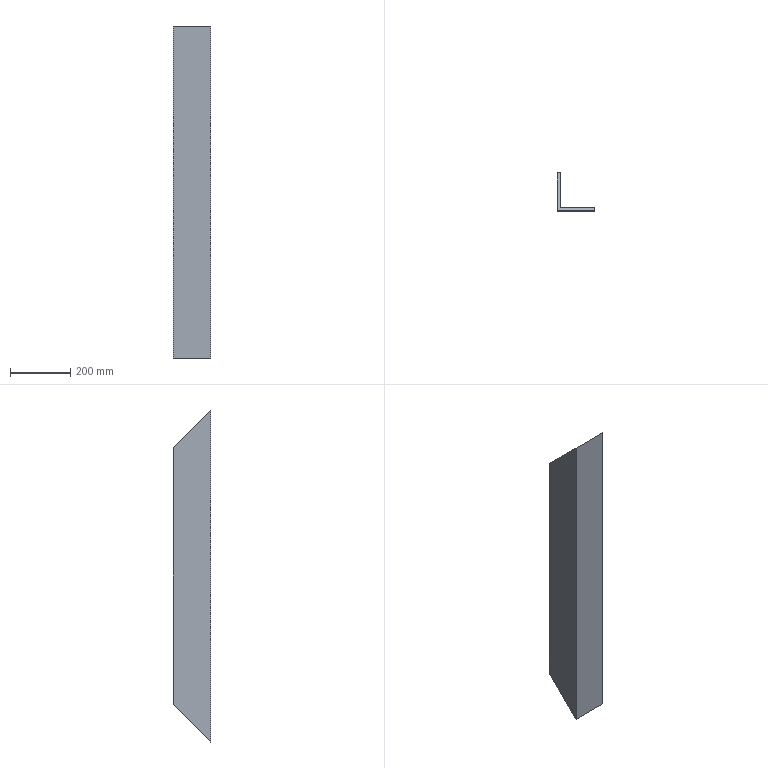Part | SolidWorks | features Extrusion 1, ICE 1 | 1 solid | 8 faces | box 125 x 125 x 1100 mm | volume 2472250 mm3 | plane 8
STEP:
#1=CARTESIAN_POINT('',(0.,125.,425.));
#2=VERTEX_POINT('',#1);
#3=CARTESIAN_POINT('',(10.,125.,425.));
#4=VERTEX_POINT('',#3);
#5=CARTESIAN_POINT('',(0.,125.,425.));
#6=DIRECTION('',(1.,0.,0.));
#7=VECTOR('',#6,1000.);
#8=LINE('',#5,#7);
#9=EDGE_CURVE('',#2,#4,#8,.T.);
#10=ORIENTED_EDGE('',*,*,#9,.T.);
#11=CARTESIAN_POINT('',(10.,125.,-425.));
#12=VERTEX_POINT('',#11);
#13=CARTESIAN_POINT('',(10.,125.,550.));
#14=DIRECTION('',(0.,0.,-1.));
#15=VECTOR('',#14,1000.);
#16=LINE('',#13,#15);
#17=EDGE_CURVE('',#4,#12,#16,.T.);
#18=ORIENTED_EDGE('',*,*,#17,.T.);
#19=CARTESIAN_POINT('',(0.,125.,-425.));
#20=VERTEX_POINT('',#19);
#21=CARTESIAN_POINT('',(0.,125.,-425.));
#22=DIRECTION('',(1.,0.,0.));
#23=VECTOR('',#22,1000.);
#24=LINE('',#21,#23);
#25=EDGE_CURVE('',#20,#12,#24,.T.);
#26=ORIENTED_EDGE('',*,*,#25,.F.);
#27=CARTESIAN_POINT('',(0.,125.,550.));
#28=DIRECTION('',(0.,0.,-1.));
#29=VECTOR('',#28,1000.);
#30=LINE('',#27,#29);
#31=EDGE_CURVE('',#2,#20,#30,.T.);
#32=ORIENTED_EDGE('',*,*,#31,.F.);
#33=EDGE_LOOP('',(#10,#18,#26,#32));
#34=FACE_OUTER_BOUND('',#33,.T.);
#35=CARTESIAN_POINT('',(0.,125.,550.));
#36=DIRECTION('',(0.,1.,0.));
#37=DIRECTION('',(0.,0.,1.));
#38=AXIS2_PLACEMENT_3D('',#35,#36,#37);
#39=PLANE('',#38);
#40=ADVANCED_FACE('',(#34),#39,.T.);
#41=CARTESIAN_POINT('',(0.,0.,550.));
#42=VERTEX_POINT('',#41);
#43=CARTESIAN_POINT('',(0.,0.,-550.));
#44=VERTEX_POINT('',#43);
#45=CARTESIAN_POINT('',(0.,0.,550.));
#46=DIRECTION('',(0.,0.,-1.));
#47=VECTOR('',#46,1000.);
#48=LINE('',#45,#47);
#49=EDGE_CURVE('',#42,#44,#48,.T.);
#50=ORIENTED_EDGE('',*,*,#49,.F.);
#51=CARTESIAN_POINT('',(0.,125.,425.));
#52=DIRECTION('',(0.,0.7071,-0.7071));
#53=VECTOR('',#52,1000.);
#54=LINE('',#51,#53);
#55=EDGE_CURVE('',#42,#2,#54,.T.);
#56=ORIENTED_EDGE('',*,*,#55,.T.);
#57=ORIENTED_EDGE('',*,*,#31,.T.);
#58=CARTESIAN_POINT('',(0.,125.,-425.));
#59=DIRECTION('',(0.,-0.7071,-0.7071));
#60=VECTOR('',#59,1000.);
#61=LINE('',#58,#60);
#62=EDGE_CURVE('',#20,#44,#61,.T.);
#63=ORIENTED_EDGE('',*,*,#62,.T.);
#64=EDGE_LOOP('',(#50,#56,#57,#63));
#65=FACE_OUTER_BOUND('',#64,.T.);
#66=CARTESIAN_POINT('',(0.,0.,550.));
#67=DIRECTION('',(1.,0.,0.));
#68=DIRECTION('',(0.,1.,0.));
#69=AXIS2_PLACEMENT_3D('',#66,#67,#68);
#70=PLANE('',#69);
#71=ADVANCED_FACE('',(#65),#70,.F.);
#72=CARTESIAN_POINT('',(125.,0.,-550.));
#73=VERTEX_POINT('',#72);
#74=CARTESIAN_POINT('',(0.,0.,-550.));
#75=DIRECTION('',(1.,0.,0.));
#76=VECTOR('',#75,1000.);
#77=LINE('',#74,#76);
#78=EDGE_CURVE('',#44,#73,#77,.T.);
#79=ORIENTED_EDGE('',*,*,#78,.T.);
#80=CARTESIAN_POINT('',(125.,0.,550.));
#81=VERTEX_POINT('',#80);
#82=CARTESIAN_POINT('',(125.,0.,550.));
#83=DIRECTION('',(0.,0.,-1.));
#84=VECTOR('',#83,1000.);
#85=LINE('',#82,#84);
#86=EDGE_CURVE('',#81,#73,#85,.T.);
#87=ORIENTED_EDGE('',*,*,#86,.F.);
#88=CARTESIAN_POINT('',(0.,0.,550.));
#89=DIRECTION('',(1.,0.,0.));
#90=VECTOR('',#89,1000.);
#91=LINE('',#88,#90);
#92=EDGE_CURVE('',#42,#81,#91,.T.);
#93=ORIENTED_EDGE('',*,*,#92,.F.);
#94=ORIENTED_EDGE('',*,*,#49,.T.);
#95=EDGE_LOOP('',(#79,#87,#93,#94));
#96=FACE_OUTER_BOUND('',#95,.T.);
#97=CARTESIAN_POINT('',(0.,0.,550.));
#98=DIRECTION('',(0.,1.,0.));
#99=DIRECTION('',(0.,0.,1.));
#100=AXIS2_PLACEMENT_3D('',#97,#98,#99);
#101=PLANE('',#100);
#102=ADVANCED_FACE('',(#96),#101,.F.);
#103=CARTESIAN_POINT('',(125.,10.,540.));
#104=VERTEX_POINT('',#103);
#105=CARTESIAN_POINT('',(125.,10.,-540.));
#106=VERTEX_POINT('',#105);
#107=CARTESIAN_POINT('',(125.,10.,550.));
#108=DIRECTION('',(0.,0.,-1.));
#109=VECTOR('',#108,1000.);
#110=LINE('',#107,#109);
#111=EDGE_CURVE('',#104,#106,#110,.T.);
#112=ORIENTED_EDGE('',*,*,#111,.F.);
#113=CARTESIAN_POINT('',(125.,125.,425.));
#114=DIRECTION('',(0.,0.7071,-0.7071));
#115=VECTOR('',#114,1000.);
#116=LINE('',#113,#115);
#117=EDGE_CURVE('',#81,#104,#116,.T.);
#118=ORIENTED_EDGE('',*,*,#117,.F.);
#119=ORIENTED_EDGE('',*,*,#86,.T.);
#120=CARTESIAN_POINT('',(125.,125.,-425.));
#121=DIRECTION('',(0.,-0.7071,-0.7071));
#122=VECTOR('',#121,1000.);
#123=LINE('',#120,#122);
#124=EDGE_CURVE('',#106,#73,#123,.T.);
#125=ORIENTED_EDGE('',*,*,#124,.F.);
#126=EDGE_LOOP('',(#112,#118,#119,#125));
#127=FACE_OUTER_BOUND('',#126,.T.);
#128=CARTESIAN_POINT('',(125.,0.,550.));
#129=DIRECTION('',(-1.,0.,0.));
#130=DIRECTION('',(0.,0.,1.));
#131=AXIS2_PLACEMENT_3D('',#128,#129,#130);
#132=PLANE('',#131);
#133=ADVANCED_FACE('',(#127),#132,.F.);
#134=CARTESIAN_POINT('',(10.,10.,540.));
#135=VERTEX_POINT('',#134);
#136=CARTESIAN_POINT('',(0.,10.,540.));
#137=DIRECTION('',(-1.,0.,0.));
#138=VECTOR('',#137,1000.);
#139=LINE('',#136,#138);
#140=EDGE_CURVE('',#104,#135,#139,.T.);
#141=ORIENTED_EDGE('',*,*,#140,.F.);
#142=ORIENTED_EDGE('',*,*,#111,.T.);
#143=CARTESIAN_POINT('',(10.,10.,-540.));
#144=VERTEX_POINT('',#143);
#145=CARTESIAN_POINT('',(0.,10.,-540.));
#146=DIRECTION('',(1.,0.,0.));
#147=VECTOR('',#146,1000.);
#148=LINE('',#145,#147);
#149=EDGE_CURVE('',#144,#106,#148,.T.);
#150=ORIENTED_EDGE('',*,*,#149,.F.);
#151=CARTESIAN_POINT('',(10.,10.,550.));
#152=DIRECTION('',(0.,0.,-1.));
#153=VECTOR('',#152,1000.);
#154=LINE('',#151,#153);
#155=EDGE_CURVE('',#135,#144,#154,.T.);
#156=ORIENTED_EDGE('',*,*,#155,.F.);
#157=EDGE_LOOP('',(#141,#142,#150,#156));
#158=FACE_OUTER_BOUND('',#157,.T.);
#159=CARTESIAN_POINT('',(0.,10.,550.));
#160=DIRECTION('',(0.,1.,0.));
#161=DIRECTION('',(0.,0.,1.));
#162=AXIS2_PLACEMENT_3D('',#159,#160,#161);
#163=PLANE('',#162);
#164=ADVANCED_FACE('',(#158),#163,.T.);
#165=CARTESIAN_POINT('',(10.,0.,550.));
#166=DIRECTION('',(0.,0.7071,-0.7071));
#167=VECTOR('',#166,1000.);
#168=LINE('',#165,#167);
#169=EDGE_CURVE('',#135,#4,#168,.T.);
#170=ORIENTED_EDGE('',*,*,#169,.F.);
#171=ORIENTED_EDGE('',*,*,#155,.T.);
#172=CARTESIAN_POINT('',(10.,550.,0.));
#173=DIRECTION('',(0.,-0.7071,-0.7071));
#174=VECTOR('',#173,1000.);
#175=LINE('',#172,#174);
#176=EDGE_CURVE('',#12,#144,#175,.T.);
#177=ORIENTED_EDGE('',*,*,#176,.F.);
#178=ORIENTED_EDGE('',*,*,#17,.F.);
#179=EDGE_LOOP('',(#170,#171,#177,#178));
#180=FACE_OUTER_BOUND('',#179,.T.);
#181=CARTESIAN_POINT('',(10.,0.,550.));
#182=DIRECTION('',(1.,0.,0.));
#183=DIRECTION('',(0.,1.,0.));
#184=AXIS2_PLACEMENT_3D('',#181,#182,#183);
#185=PLANE('',#184);
#186=ADVANCED_FACE('',(#180),#185,.T.);
#187=ORIENTED_EDGE('',*,*,#149,.T.);
#188=ORIENTED_EDGE('',*,*,#124,.T.);
#189=ORIENTED_EDGE('',*,*,#78,.F.);
#190=ORIENTED_EDGE('',*,*,#62,.F.);
#191=ORIENTED_EDGE('',*,*,#25,.T.);
#192=ORIENTED_EDGE('',*,*,#176,.T.);
#193=EDGE_LOOP('',(#187,#188,#189,#190,#191,#192));
#194=FACE_OUTER_BOUND('',#193,.T.);
#195=CARTESIAN_POINT('',(0.,125.,-425.));
#196=DIRECTION('',(0.,-0.7071,0.7071));
#197=DIRECTION('',(0.,-0.7071,-0.7071));
#198=AXIS2_PLACEMENT_3D('',#195,#196,#197);
#199=PLANE('',#198);
#200=ADVANCED_FACE('',(#194),#199,.F.);
#201=ORIENTED_EDGE('',*,*,#140,.T.);
#202=ORIENTED_EDGE('',*,*,#169,.T.);
#203=ORIENTED_EDGE('',*,*,#9,.F.);
#204=ORIENTED_EDGE('',*,*,#55,.F.);
#205=ORIENTED_EDGE('',*,*,#92,.T.);
#206=ORIENTED_EDGE('',*,*,#117,.T.);
#207=EDGE_LOOP('',(#201,#202,#203,#204,#205,#206));
#208=FACE_OUTER_BOUND('',#207,.T.);
#209=CARTESIAN_POINT('',(0.,125.,425.));
#210=DIRECTION('',(0.,-0.7071,-0.7071));
#211=DIRECTION('',(0.,0.7071,-0.7071));
#212=AXIS2_PLACEMENT_3D('',#209,#210,#211);
#213=PLANE('',#212);
#214=ADVANCED_FACE('',(#208),#213,.F.);
#215=CLOSED_SHELL('',(#40,#71,#102,#133,#164,#186,#200,#214));
#216=MANIFOLD_SOLID_BREP('',#215);
#217=CARTESIAN_POINT('',(0.,0.,0.));
#218=DIRECTION('',(0.,0.,1.));
#219=DIRECTION('',(1.,0.,0.));
#220=AXIS2_PLACEMENT_3D('',#217,#218,#219);
#221=(LENGTH_UNIT()NAMED_UNIT(*)SI_UNIT(.MILLI.,.METRE.));
#222=UNCERTAINTY_MEASURE_WITH_UNIT(LENGTH_MEASURE(0.00001),#221,'','');
#223=(NAMED_UNIT(*)PLANE_ANGLE_UNIT()SI_UNIT($,.RADIAN.));
#224=(NAMED_UNIT(*)SI_UNIT($,.STERADIAN.)SOLID_ANGLE_UNIT());
#225=(GEOMETRIC_REPRESENTATION_CONTEXT(3)GLOBAL_UNCERTAINTY_ASSIGNED_CONTEXT((#222))GLOBAL_UNIT_ASSIGNED_CONTEXT((#221,#223,#224))REPRESENTATION_CONTEXT('',''));
#226=ADVANCED_BREP_SHAPE_REPRESENTATION('',(#216,#220),#225);